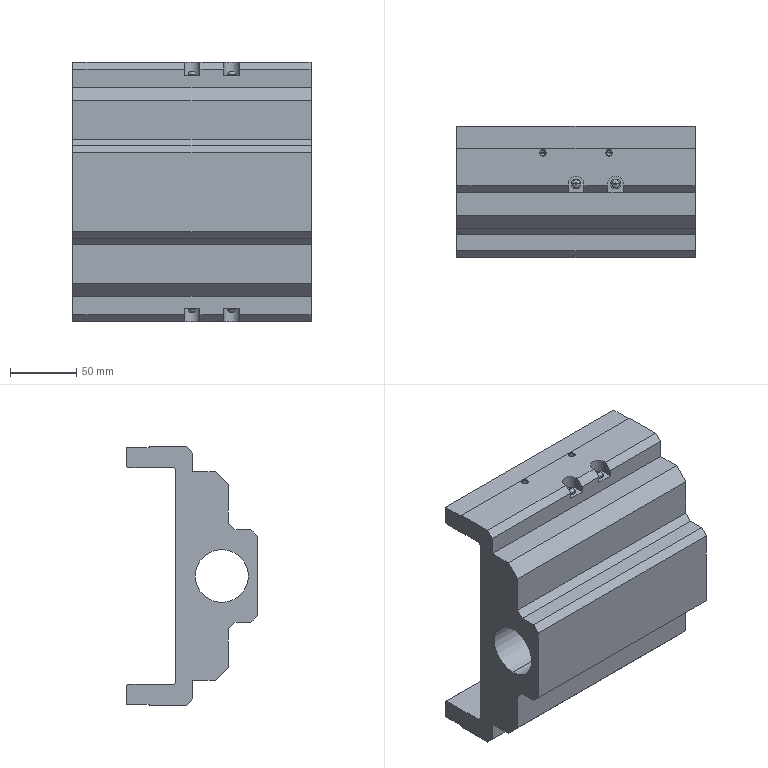Part | STEP file | ISB-WXMX-WA-750-25-1500-T4-N-A1-AQ-EB-^-Part-2 | 1 solid | 186 faces | box 180 x 99 x 196 mm | volume 1445852 mm3 | cylinder 68 | plane 62 | cone 48 | other 8 | commonest cylinder face diameters 6.647 x16 8 x12 4.134 x8 6 x8 6.9 x8 7.5 x8